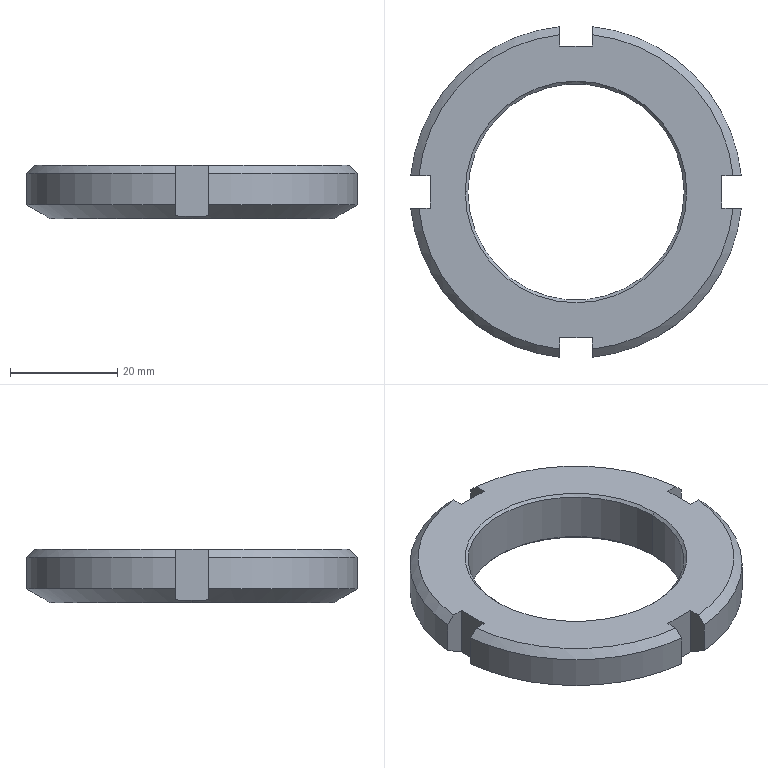Part | SolidWorks | features Chamfer 3, CirPattern 1, Cut 1, Extrusion 1 | 1 solid | 30 faces | box 61.709 x 61.709 x 10 mm | volume 15331 mm3 | plane 14 | cone 10 | cylinder 6 | commonest cylinder face diameters 62 x4 40.376 x2
STEP:
#1=CARTESIAN_POINT('',(-20.188,0.,9.5));
#2=VERTEX_POINT('',#1);
#3=CARTESIAN_POINT('',(20.188,0.,9.5));
#4=VERTEX_POINT('',#3);
#5=CARTESIAN_POINT('',(0.,0.,9.5));
#6=DIRECTION('',(0.,0.,1.));
#7=DIRECTION('',(1.,0.,0.));
#8=AXIS2_PLACEMENT_3D('',#5,#6,#7);
#9=CIRCLE('',#8,20.188);
#10=EDGE_CURVE('',#2,#4,#9,.T.);
#11=ORIENTED_EDGE('',*,*,#10,.F.);
#12=CARTESIAN_POINT('',(-20.688,0.,10.));
#13=VERTEX_POINT('',#12);
#14=CARTESIAN_POINT('',(-20.188,0.,9.5));
#15=DIRECTION('',(-0.7071,0.,0.7071));
#16=VECTOR('',#15,1000.);
#17=LINE('',#14,#16);
#18=EDGE_CURVE('',#2,#13,#17,.T.);
#19=ORIENTED_EDGE('',*,*,#18,.T.);
#20=CARTESIAN_POINT('',(20.688,0.,10.));
#21=VERTEX_POINT('',#20);
#22=CARTESIAN_POINT('',(0.,0.,10.));
#23=DIRECTION('',(0.,0.,-1.));
#24=DIRECTION('',(1.,0.,0.));
#25=AXIS2_PLACEMENT_3D('',#22,#23,#24);
#26=CIRCLE('',#25,20.688);
#27=EDGE_CURVE('',#21,#13,#26,.T.);
#28=ORIENTED_EDGE('',*,*,#27,.F.);
#29=CARTESIAN_POINT('',(20.188,0.,9.5));
#30=DIRECTION('',(0.7071,0.,0.7071));
#31=VECTOR('',#30,1000.);
#32=LINE('',#29,#31);
#33=EDGE_CURVE('',#4,#21,#32,.T.);
#34=ORIENTED_EDGE('',*,*,#33,.F.);
#35=EDGE_LOOP('',(#11,#19,#28,#34));
#36=FACE_OUTER_BOUND('',#35,.T.);
#37=CARTESIAN_POINT('',(0.,0.,9.5));
#38=DIRECTION('',(0.,0.,1.));
#39=DIRECTION('',(1.,0.,0.));
#40=AXIS2_PLACEMENT_3D('',#37,#38,#39);
#41=CONICAL_SURFACE('',#40,20.188,0.7854);
#42=ADVANCED_FACE('',(#36),#41,.F.);
#43=CARTESIAN_POINT('',(20.188,0.,0.5));
#44=VERTEX_POINT('',#43);
#45=CARTESIAN_POINT('',(-20.188,0.,0.5));
#46=VERTEX_POINT('',#45);
#47=CARTESIAN_POINT('',(0.,0.,0.5));
#48=DIRECTION('',(0.,0.,-1.));
#49=DIRECTION('',(1.,0.,0.));
#50=AXIS2_PLACEMENT_3D('',#47,#48,#49);
#51=CIRCLE('',#50,20.188);
#52=EDGE_CURVE('',#44,#46,#51,.T.);
#53=ORIENTED_EDGE('',*,*,#52,.F.);
#54=CARTESIAN_POINT('',(20.688,0.,0.));
#55=VERTEX_POINT('',#54);
#56=CARTESIAN_POINT('',(20.688,0.,0.));
#57=DIRECTION('',(0.7071,0.,-0.7071));
#58=VECTOR('',#57,1000.);
#59=LINE('',#56,#58);
#60=EDGE_CURVE('',#44,#55,#59,.T.);
#61=ORIENTED_EDGE('',*,*,#60,.T.);
#62=CARTESIAN_POINT('',(-20.688,0.,0.));
#63=VERTEX_POINT('',#62);
#64=CARTESIAN_POINT('',(0.,0.,0.));
#65=DIRECTION('',(0.,0.,1.));
#66=DIRECTION('',(1.,0.,0.));
#67=AXIS2_PLACEMENT_3D('',#64,#65,#66);
#68=CIRCLE('',#67,20.688);
#69=EDGE_CURVE('',#63,#55,#68,.T.);
#70=ORIENTED_EDGE('',*,*,#69,.F.);
#71=CARTESIAN_POINT('',(-20.688,0.,0.));
#72=DIRECTION('',(-0.7071,0.,-0.7071));
#73=VECTOR('',#72,1000.);
#74=LINE('',#71,#73);
#75=EDGE_CURVE('',#46,#63,#74,.T.);
#76=ORIENTED_EDGE('',*,*,#75,.F.);
#77=EDGE_LOOP('',(#53,#61,#70,#76));
#78=FACE_OUTER_BOUND('',#77,.T.);
#79=CARTESIAN_POINT('',(0.,0.,0.));
#80=DIRECTION('',(0.,0.,-1.));
#81=DIRECTION('',(-1.,0.,0.));
#82=AXIS2_PLACEMENT_3D('',#79,#80,#81);
#83=CONICAL_SURFACE('',#82,20.688,0.7854);
#84=ADVANCED_FACE('',(#78),#83,.F.);
#85=CARTESIAN_POINT('',(-26.5,0.,0.));
#86=VERTEX_POINT('',#85);
#87=CARTESIAN_POINT('',(26.5,0.,0.));
#88=VERTEX_POINT('',#87);
#89=CARTESIAN_POINT('',(0.,0.,0.));
#90=DIRECTION('',(0.,0.,-1.));
#91=DIRECTION('',(1.,0.,0.));
#92=AXIS2_PLACEMENT_3D('',#89,#90,#91);
#93=CIRCLE('',#92,26.5);
#94=EDGE_CURVE('',#86,#88,#93,.T.);
#95=ORIENTED_EDGE('',*,*,#94,.F.);
#96=CARTESIAN_POINT('',(-27.254,0.,0.4356));
#97=VERTEX_POINT('',#96);
#98=CARTESIAN_POINT('',(-31.,0.,2.598));
#99=DIRECTION('',(-0.866,0.,0.5));
#100=VECTOR('',#99,1000.);
#101=LINE('',#98,#100);
#102=EDGE_CURVE('',#86,#97,#101,.T.);
#103=ORIENTED_EDGE('',*,*,#102,.T.);
#104=CARTESIAN_POINT('',(-27.254,3.,0.5306));
#105=VERTEX_POINT('',#104);
#106=CARTESIAN_POINT('',(-27.254,3.,0.5306));
#107=CARTESIAN_POINT('',(-27.254,2.003,0.4677));
#108=CARTESIAN_POINT('',(-27.254,1.003,0.4356));
#109=CARTESIAN_POINT('',(-27.254,0.,0.4356));
#110=B_SPLINE_CURVE_WITH_KNOTS('',3,(#106,#107,#108,#109),.UNSPECIFIED.,.F.,.F.,(4,4),(0.007971,0.01097),.UNSPECIFIED.);
#111=EDGE_CURVE('',#105,#97,#110,.T.);
#112=ORIENTED_EDGE('',*,*,#111,.F.);
#113=CARTESIAN_POINT('',(-30.854,3.,2.598));
#114=VERTEX_POINT('',#113);
#115=CARTESIAN_POINT('',(-30.854,3.,2.598));
#116=CARTESIAN_POINT('',(-30.648,3.,2.48));
#117=CARTESIAN_POINT('',(-30.442,3.,2.361));
#118=CARTESIAN_POINT('',(-30.236,3.,2.242));
#119=CARTESIAN_POINT('',(-29.242,3.,1.672));
#120=CARTESIAN_POINT('',(-28.248,3.,1.101));
#121=CARTESIAN_POINT('',(-27.254,3.,0.5306));
#122=B_SPLINE_CURVE_WITH_KNOTS('',3,(#115,#116,#117,#118,#119,#120,#121),.UNSPECIFIED.,.F.,.F.,(4,3,4),(0.007772,0.008485,0.01192),.UNSPECIFIED.);
#123=EDGE_CURVE('',#114,#105,#122,.T.);
#124=ORIENTED_EDGE('',*,*,#123,.F.);
#125=CARTESIAN_POINT('',(-3.,30.854,2.598));
#126=VERTEX_POINT('',#125);
#127=CARTESIAN_POINT('',(0.,0.,2.598));
#128=DIRECTION('',(0.,0.,1.));
#129=DIRECTION('',(1.,0.,0.));
#130=AXIS2_PLACEMENT_3D('',#127,#128,#129);
#131=CIRCLE('',#130,31.);
#132=EDGE_CURVE('',#126,#114,#131,.T.);
#133=ORIENTED_EDGE('',*,*,#132,.F.);
#134=CARTESIAN_POINT('',(-3.,27.254,0.5306));
#135=VERTEX_POINT('',#134);
#136=CARTESIAN_POINT('',(-3.,27.254,0.5306));
#137=CARTESIAN_POINT('',(-3.,28.455,1.219));
#138=CARTESIAN_POINT('',(-3.,29.655,1.909));
#139=CARTESIAN_POINT('',(-3.,30.854,2.598));
#140=B_SPLINE_CURVE_WITH_KNOTS('',3,(#136,#137,#138,#139),.UNSPECIFIED.,.F.,.F.,(4,4),(0.008036,0.01219),.UNSPECIFIED.);
#141=EDGE_CURVE('',#135,#126,#140,.T.);
#142=ORIENTED_EDGE('',*,*,#141,.F.);
#143=CARTESIAN_POINT('',(3.,27.254,0.5306));
#144=VERTEX_POINT('',#143);
#145=CARTESIAN_POINT('',(3.,27.254,0.5306));
#146=CARTESIAN_POINT('',(2.005,27.254,0.4678));
#147=CARTESIAN_POINT('',(1.008,27.254,0.4358));
#148=CARTESIAN_POINT('',(-0.9926,27.254,0.4354));
#149=CARTESIAN_POINT('',(-1.998,27.254,0.4674));
#150=CARTESIAN_POINT('',(-3.,27.254,0.5306));
#151=B_SPLINE_CURVE_WITH_KNOTS('',3,(#145,#146,#147,#148,#149,#150),.UNSPECIFIED.,.F.,.F.,(4,2,4),(0.007971,0.01096,0.01395),.UNSPECIFIED.);
#152=EDGE_CURVE('',#144,#135,#151,.T.);
#153=ORIENTED_EDGE('',*,*,#152,.F.);
#154=CARTESIAN_POINT('',(3.,30.854,2.598));
#155=VERTEX_POINT('',#154);
#156=CARTESIAN_POINT('',(3.,30.854,2.598));
#157=CARTESIAN_POINT('',(3.,29.655,1.909));
#158=CARTESIAN_POINT('',(3.,28.455,1.219));
#159=CARTESIAN_POINT('',(3.,27.254,0.5306));
#160=B_SPLINE_CURVE_WITH_KNOTS('',3,(#156,#157,#158,#159),.UNSPECIFIED.,.F.,.F.,(4,4),(0.004783,0.008935),.UNSPECIFIED.);
#161=EDGE_CURVE('',#155,#144,#160,.T.);
#162=ORIENTED_EDGE('',*,*,#161,.F.);
#163=CARTESIAN_POINT('',(30.854,3.,2.598));
#164=VERTEX_POINT('',#163);
#165=CARTESIAN_POINT('',(0.,0.,2.598));
#166=DIRECTION('',(0.,0.,1.));
#167=DIRECTION('',(1.,0.,0.));
#168=AXIS2_PLACEMENT_3D('',#165,#166,#167);
#169=CIRCLE('',#168,31.);
#170=EDGE_CURVE('',#164,#155,#169,.T.);
#171=ORIENTED_EDGE('',*,*,#170,.F.);
#172=CARTESIAN_POINT('',(27.254,3.,0.5306));
#173=VERTEX_POINT('',#172);
#174=CARTESIAN_POINT('',(27.254,3.,0.5306));
#175=CARTESIAN_POINT('',(28.455,3.,1.219));
#176=CARTESIAN_POINT('',(29.655,3.,1.909));
#177=CARTESIAN_POINT('',(30.854,3.,2.598));
#178=B_SPLINE_CURVE_WITH_KNOTS('',3,(#174,#175,#176,#177),.UNSPECIFIED.,.F.,.F.,(4,4),(0.008036,0.01219),.UNSPECIFIED.);
#179=EDGE_CURVE('',#173,#164,#178,.T.);
#180=ORIENTED_EDGE('',*,*,#179,.F.);
#181=CARTESIAN_POINT('',(27.254,0.,0.4356));
#182=VERTEX_POINT('',#181);
#183=CARTESIAN_POINT('',(27.254,0.,0.4356));
#184=CARTESIAN_POINT('',(27.254,1.003,0.4356));
#185=CARTESIAN_POINT('',(27.254,2.003,0.4677));
#186=CARTESIAN_POINT('',(27.254,3.,0.5306));
#187=B_SPLINE_CURVE_WITH_KNOTS('',3,(#183,#184,#185,#186),.UNSPECIFIED.,.F.,.F.,(4,4),(0.01544,0.01844),.UNSPECIFIED.);
#188=EDGE_CURVE('',#182,#173,#187,.T.);
#189=ORIENTED_EDGE('',*,*,#188,.F.);
#190=CARTESIAN_POINT('',(31.,0.,2.598));
#191=DIRECTION('',(0.866,0.,0.5));
#192=VECTOR('',#191,1000.);
#193=LINE('',#190,#192);
#194=EDGE_CURVE('',#88,#182,#193,.T.);
#195=ORIENTED_EDGE('',*,*,#194,.F.);
#196=EDGE_LOOP('',(#95,#103,#112,#124,#133,#142,#153,#162,#171,#180,#189,#195));
#197=FACE_OUTER_BOUND('',#196,.T.);
#198=CARTESIAN_POINT('',(0.,0.,2.598));
#199=DIRECTION('',(0.,0.,1.));
#200=DIRECTION('',(1.,0.,0.));
#201=AXIS2_PLACEMENT_3D('',#198,#199,#200);
#202=CONICAL_SURFACE('',#201,31.,1.047);
#203=ADVANCED_FACE('',(#197),#202,.T.);
#204=ORIENTED_EDGE('',*,*,#10,.T.);
#205=CARTESIAN_POINT('',(20.188,0.,10.));
#206=DIRECTION('',(0.,0.,-1.));
#207=VECTOR('',#206,1000.);
#208=LINE('',#205,#207);
#209=EDGE_CURVE('',#4,#44,#208,.T.);
#210=ORIENTED_EDGE('',*,*,#209,.T.);
#211=ORIENTED_EDGE('',*,*,#52,.T.);
#212=CARTESIAN_POINT('',(-20.188,0.,10.));
#213=DIRECTION('',(0.,0.,-1.));
#214=VECTOR('',#213,1000.);
#215=LINE('',#212,#214);
#216=EDGE_CURVE('',#2,#46,#215,.T.);
#217=ORIENTED_EDGE('',*,*,#216,.F.);
#218=EDGE_LOOP('',(#204,#210,#211,#217));
#219=FACE_OUTER_BOUND('',#218,.T.);
#220=CARTESIAN_POINT('',(0.,0.,10.));
#221=DIRECTION('',(0.,0.,-1.));
#222=DIRECTION('',(-1.,0.,0.));
#223=AXIS2_PLACEMENT_3D('',#220,#221,#222);
#224=CYLINDRICAL_SURFACE('',#223,20.188);
#225=ADVANCED_FACE('',(#219),#224,.F.);
#226=CARTESIAN_POINT('',(3.,30.854,8.5));
#227=VERTEX_POINT('',#226);
#228=CARTESIAN_POINT('',(30.854,3.,8.5));
#229=VERTEX_POINT('',#228);
#230=CARTESIAN_POINT('',(0.,0.,8.5));
#231=DIRECTION('',(0.,0.,-1.));
#232=DIRECTION('',(1.,0.,0.));
#233=AXIS2_PLACEMENT_3D('',#230,#231,#232);
#234=CIRCLE('',#233,31.);
#235=EDGE_CURVE('',#227,#229,#234,.T.);
#236=ORIENTED_EDGE('',*,*,#235,.T.);
#237=CARTESIAN_POINT('',(30.854,3.,0.));
#238=DIRECTION('',(0.,0.,1.));
#239=VECTOR('',#238,1000.);
#240=LINE('',#237,#239);
#241=EDGE_CURVE('',#164,#229,#240,.T.);
#242=ORIENTED_EDGE('',*,*,#241,.F.);
#243=ORIENTED_EDGE('',*,*,#170,.T.);
#244=CARTESIAN_POINT('',(3.,30.854,0.));
#245=DIRECTION('',(0.,0.,1.));
#246=VECTOR('',#245,1000.);
#247=LINE('',#244,#246);
#248=EDGE_CURVE('',#155,#227,#247,.T.);
#249=ORIENTED_EDGE('',*,*,#248,.T.);
#250=EDGE_LOOP('',(#236,#242,#243,#249));
#251=FACE_OUTER_BOUND('',#250,.T.);
#252=CARTESIAN_POINT('',(0.,0.,10.));
#253=DIRECTION('',(0.,0.,-1.));
#254=DIRECTION('',(-1.,0.,0.));
#255=AXIS2_PLACEMENT_3D('',#252,#253,#254);
#256=CYLINDRICAL_SURFACE('',#255,31.);
#257=ADVANCED_FACE('',(#251),#256,.T.);
#258=CARTESIAN_POINT('',(29.347,3.,10.));
#259=VERTEX_POINT('',#258);
#260=CARTESIAN_POINT('',(30.854,3.,8.5));
#261=CARTESIAN_POINT('',(30.441,3.,8.912));
#262=CARTESIAN_POINT('',(30.027,3.,9.323));
#263=CARTESIAN_POINT('',(29.614,3.,9.735));
#264=CARTESIAN_POINT('',(29.525,3.,9.823));
#265=CARTESIAN_POINT('',(29.436,3.,9.912));
#266=CARTESIAN_POINT('',(29.347,3.,10.));
#267=B_SPLINE_CURVE_WITH_KNOTS('',3,(#260,#261,#262,#263,#264,#265,#266),.UNSPECIFIED.,.F.,.F.,(4,3,4),(0.006071,0.007821,0.008198),.UNSPECIFIED.);
#268=EDGE_CURVE('',#229,#259,#267,.T.);
#269=ORIENTED_EDGE('',*,*,#268,.F.);
#270=ORIENTED_EDGE('',*,*,#235,.F.);
#271=CARTESIAN_POINT('',(3.,29.347,10.));
#272=VERTEX_POINT('',#271);
#273=CARTESIAN_POINT('',(3.,29.347,10.));
#274=CARTESIAN_POINT('',(3.,29.436,9.912));
#275=CARTESIAN_POINT('',(3.,29.525,9.823));
#276=CARTESIAN_POINT('',(3.,29.614,9.735));
#277=CARTESIAN_POINT('',(3.,30.027,9.323));
#278=CARTESIAN_POINT('',(3.,30.441,8.912));
#279=CARTESIAN_POINT('',(3.,30.854,8.5));
#280=B_SPLINE_CURVE_WITH_KNOTS('',3,(#273,#274,#275,#276,#277,#278,#279),.UNSPECIFIED.,.F.,.F.,(4,3,4),(0.007445,0.007821,0.009572),.UNSPECIFIED.);
#281=EDGE_CURVE('',#272,#227,#280,.T.);
#282=ORIENTED_EDGE('',*,*,#281,.F.);
#283=CARTESIAN_POINT('',(0.,0.,10.));
#284=DIRECTION('',(0.,0.,1.));
#285=DIRECTION('',(1.,0.,0.));
#286=AXIS2_PLACEMENT_3D('',#283,#284,#285);
#287=CIRCLE('',#286,29.5);
#288=EDGE_CURVE('',#259,#272,#287,.T.);
#289=ORIENTED_EDGE('',*,*,#288,.F.);
#290=EDGE_LOOP('',(#269,#270,#282,#289));
#291=FACE_OUTER_BOUND('',#290,.T.);
#292=CARTESIAN_POINT('',(0.,0.,10.));
#293=DIRECTION('',(0.,0.,-1.));
#294=DIRECTION('',(-1.,0.,0.));
#295=AXIS2_PLACEMENT_3D('',#292,#293,#294);
#296=CONICAL_SURFACE('',#295,29.5,0.7854);
#297=ADVANCED_FACE('',(#291),#296,.T.);
#298=CARTESIAN_POINT('',(-30.854,3.,8.5));
#299=VERTEX_POINT('',#298);
#300=CARTESIAN_POINT('',(-3.,30.854,8.5));
#301=VERTEX_POINT('',#300);
#302=CARTESIAN_POINT('',(0.,0.,8.5));
#303=DIRECTION('',(0.,0.,-1.));
#304=DIRECTION('',(1.,0.,0.));
#305=AXIS2_PLACEMENT_3D('',#302,#303,#304);
#306=CIRCLE('',#305,31.);
#307=EDGE_CURVE('',#299,#301,#306,.T.);
#308=ORIENTED_EDGE('',*,*,#307,.T.);
#309=CARTESIAN_POINT('',(-3.,30.854,0.));
#310=DIRECTION('',(0.,0.,1.));
#311=VECTOR('',#310,1000.);
#312=LINE('',#309,#311);
#313=EDGE_CURVE('',#126,#301,#312,.T.);
#314=ORIENTED_EDGE('',*,*,#313,.F.);
#315=ORIENTED_EDGE('',*,*,#132,.T.);
#316=CARTESIAN_POINT('',(-30.854,3.,0.));
#317=DIRECTION('',(0.,0.,1.));
#318=VECTOR('',#317,1000.);
#319=LINE('',#316,#318);
#320=EDGE_CURVE('',#114,#299,#319,.T.);
#321=ORIENTED_EDGE('',*,*,#320,.T.);
#322=EDGE_LOOP('',(#308,#314,#315,#321));
#323=FACE_OUTER_BOUND('',#322,.T.);
#324=CARTESIAN_POINT('',(0.,0.,10.));
#325=DIRECTION('',(0.,0.,-1.));
#326=DIRECTION('',(-1.,0.,0.));
#327=AXIS2_PLACEMENT_3D('',#324,#325,#326);
#328=CYLINDRICAL_SURFACE('',#327,31.);
#329=ADVANCED_FACE('',(#323),#328,.T.);
#330=CARTESIAN_POINT('',(-3.,29.347,10.));
#331=VERTEX_POINT('',#330);
#332=CARTESIAN_POINT('',(-3.,30.854,8.5));
#333=CARTESIAN_POINT('',(-3.,30.441,8.912));
#334=CARTESIAN_POINT('',(-3.,30.027,9.323));
#335=CARTESIAN_POINT('',(-3.,29.614,9.735));
#336=CARTESIAN_POINT('',(-3.,29.525,9.823));
#337=CARTESIAN_POINT('',(-3.,29.436,9.912));
#338=CARTESIAN_POINT('',(-3.,29.347,10.));
#339=B_SPLINE_CURVE_WITH_KNOTS('',3,(#332,#333,#334,#335,#336,#337,#338),.UNSPECIFIED.,.F.,.F.,(4,3,4),(0.006071,0.007821,0.008198),.UNSPECIFIED.);
#340=EDGE_CURVE('',#301,#331,#339,.T.);
#341=ORIENTED_EDGE('',*,*,#340,.F.);
#342=ORIENTED_EDGE('',*,*,#307,.F.);
#343=CARTESIAN_POINT('',(-29.347,3.,10.));
#344=VERTEX_POINT('',#343);
#345=CARTESIAN_POINT('',(-29.347,3.,10.));
#346=CARTESIAN_POINT('',(-29.712,3.,9.637));
#347=CARTESIAN_POINT('',(-30.076,3.,9.274));
#348=CARTESIAN_POINT('',(-30.441,3.,8.912));
#349=CARTESIAN_POINT('',(-30.579,3.,8.774));
#350=CARTESIAN_POINT('',(-30.717,3.,8.637));
#351=CARTESIAN_POINT('',(-30.854,3.,8.5));
#352=B_SPLINE_CURVE_WITH_KNOTS('',3,(#345,#346,#347,#348,#349,#350,#351),.UNSPECIFIED.,.F.,.F.,(4,3,4),(0.006278,0.007821,0.008405),.UNSPECIFIED.);
#353=EDGE_CURVE('',#344,#299,#352,.T.);
#354=ORIENTED_EDGE('',*,*,#353,.F.);
#355=CARTESIAN_POINT('',(0.,0.,10.));
#356=DIRECTION('',(0.,0.,1.));
#357=DIRECTION('',(1.,0.,0.));
#358=AXIS2_PLACEMENT_3D('',#355,#356,#357);
#359=CIRCLE('',#358,29.5);
#360=EDGE_CURVE('',#331,#344,#359,.T.);
#361=ORIENTED_EDGE('',*,*,#360,.F.);
#362=EDGE_LOOP('',(#341,#342,#354,#361));
#363=FACE_OUTER_BOUND('',#362,.T.);
#364=CARTESIAN_POINT('',(0.,0.,10.));
#365=DIRECTION('',(0.,0.,-1.));
#366=DIRECTION('',(-1.,0.,0.));
#367=AXIS2_PLACEMENT_3D('',#364,#365,#366);
#368=CONICAL_SURFACE('',#367,29.5,0.7854);
#369=ADVANCED_FACE('',(#363),#368,.T.);
#370=CARTESIAN_POINT('',(-3.,-30.854,8.5));
#371=VERTEX_POINT('',#370);
#372=CARTESIAN_POINT('',(-30.854,-3.,8.5));
#373=VERTEX_POINT('',#372);
#374=CARTESIAN_POINT('',(0.,0.,8.5));
#375=DIRECTION('',(0.,0.,-1.));
#376=DIRECTION('',(1.,0.,0.));
#377=AXIS2_PLACEMENT_3D('',#374,#375,#376);
#378=CIRCLE('',#377,31.);
#379=EDGE_CURVE('',#371,#373,#378,.T.);
#380=ORIENTED_EDGE('',*,*,#379,.T.);
#381=CARTESIAN_POINT('',(-30.854,-3.,2.598));
#382=VERTEX_POINT('',#381);
#383=CARTESIAN_POINT('',(-30.854,-3.,0.));
#384=DIRECTION('',(0.,0.,1.));
#385=VECTOR('',#384,1000.);
#386=LINE('',#383,#385);
#387=EDGE_CURVE('',#382,#373,#386,.T.);
#388=ORIENTED_EDGE('',*,*,#387,.F.);
#389=CARTESIAN_POINT('',(-3.,-30.854,2.598));
#390=VERTEX_POINT('',#389);
#391=CARTESIAN_POINT('',(0.,0.,2.598));
#392=DIRECTION('',(0.,0.,1.));
#393=DIRECTION('',(1.,0.,0.));
#394=AXIS2_PLACEMENT_3D('',#391,#392,#393);
#395=CIRCLE('',#394,31.);
#396=EDGE_CURVE('',#382,#390,#395,.T.);
#397=ORIENTED_EDGE('',*,*,#396,.T.);
#398=CARTESIAN_POINT('',(-3.,-30.854,0.));
#399=DIRECTION('',(0.,0.,1.));
#400=VECTOR('',#399,1000.);
#401=LINE('',#398,#400);
#402=EDGE_CURVE('',#390,#371,#401,.T.);
#403=ORIENTED_EDGE('',*,*,#402,.T.);
#404=EDGE_LOOP('',(#380,#388,#397,#403));
#405=FACE_OUTER_BOUND('',#404,.T.);
#406=CARTESIAN_POINT('',(0.,0.,10.));
#407=DIRECTION('',(0.,0.,-1.));
#408=DIRECTION('',(-1.,0.,0.));
#409=AXIS2_PLACEMENT_3D('',#406,#407,#408);
#410=CYLINDRICAL_SURFACE('',#409,31.);
#411=ADVANCED_FACE('',(#405),#410,.T.);
#412=CARTESIAN_POINT('',(-29.347,-3.,10.));
#413=VERTEX_POINT('',#412);
#414=CARTESIAN_POINT('',(-30.854,-3.,8.5));
#415=CARTESIAN_POINT('',(-30.717,-3.,8.637));
#416=CARTESIAN_POINT('',(-30.579,-3.,8.774));
#417=CARTESIAN_POINT('',(-30.441,-3.,8.912));
#418=CARTESIAN_POINT('',(-30.076,-3.,9.274));
#419=CARTESIAN_POINT('',(-29.712,-3.,9.637));
#420=CARTESIAN_POINT('',(-29.347,-3.,10.));
#421=B_SPLINE_CURVE_WITH_KNOTS('',3,(#414,#415,#416,#417,#418,#419,#420),.UNSPECIFIED.,.F.,.F.,(4,3,4),(0.007238,0.007821,0.009365),.UNSPECIFIED.);
#422=EDGE_CURVE('',#373,#413,#421,.T.);
#423=ORIENTED_EDGE('',*,*,#422,.F.);
#424=ORIENTED_EDGE('',*,*,#379,.F.);
#425=CARTESIAN_POINT('',(-3.,-29.347,10.));
#426=VERTEX_POINT('',#425);
#427=CARTESIAN_POINT('',(-3.,-29.347,10.));
#428=CARTESIAN_POINT('',(-3.,-29.712,9.637));
#429=CARTESIAN_POINT('',(-3.,-30.076,9.274));
#430=CARTESIAN_POINT('',(-3.,-30.441,8.912));
#431=CARTESIAN_POINT('',(-3.,-30.579,8.774));
#432=CARTESIAN_POINT('',(-3.,-30.717,8.637));
#433=CARTESIAN_POINT('',(-3.,-30.854,8.5));
#434=B_SPLINE_CURVE_WITH_KNOTS('',3,(#427,#428,#429,#430,#431,#432,#433),.UNSPECIFIED.,.F.,.F.,(4,3,4),(0.006278,0.007821,0.008405),.UNSPECIFIED.);
#435=EDGE_CURVE('',#426,#371,#434,.T.);
#436=ORIENTED_EDGE('',*,*,#435,.F.);
#437=CARTESIAN_POINT('',(0.,0.,10.));
#438=DIRECTION('',(0.,0.,1.));
#439=DIRECTION('',(1.,0.,0.));
#440=AXIS2_PLACEMENT_3D('',#437,#438,#439);
#441=CIRCLE('',#440,29.5);
#442=EDGE_CURVE('',#413,#426,#441,.T.);
#443=ORIENTED_EDGE('',*,*,#442,.F.);
#444=EDGE_LOOP('',(#423,#424,#436,#443));
#445=FACE_OUTER_BOUND('',#444,.T.);
#446=CARTESIAN_POINT('',(0.,0.,10.));
#447=DIRECTION('',(0.,0.,-1.));
#448=DIRECTION('',(-1.,0.,0.));
#449=AXIS2_PLACEMENT_3D('',#446,#447,#448);
#450=CONICAL_SURFACE('',#449,29.5,0.7854);
#451=ADVANCED_FACE('',(#445),#450,.T.);
#452=ORIENTED_EDGE('',*,*,#27,.T.);
#453=CARTESIAN_POINT('',(0.,0.,10.));
#454=DIRECTION('',(0.,0.,-1.));
#455=DIRECTION('',(1.,0.,0.));
#456=AXIS2_PLACEMENT_3D('',#453,#454,#455);
#457=CIRCLE('',#456,20.688);
#458=EDGE_CURVE('',#13,#21,#457,.T.);
#459=ORIENTED_EDGE('',*,*,#458,.T.);
#460=EDGE_LOOP('',(#452,#459));
#461=FACE_BOUND('',#460,.T.);
#462=CARTESIAN_POINT('',(27.254,3.,10.));
#463=VERTEX_POINT('',#462);
#464=CARTESIAN_POINT('',(27.254,3.,10.));
#465=DIRECTION('',(-1.,0.,0.));
#466=VECTOR('',#465,1000.);
#467=LINE('',#464,#466);
#468=EDGE_CURVE('',#259,#463,#467,.T.);
#469=ORIENTED_EDGE('',*,*,#468,.F.);
#470=ORIENTED_EDGE('',*,*,#288,.T.);
#471=CARTESIAN_POINT('',(3.,27.254,10.));
#472=VERTEX_POINT('',#471);
#473=CARTESIAN_POINT('',(3.,27.254,10.));
#474=DIRECTION('',(0.,1.,0.));
#475=VECTOR('',#474,1000.);
#476=LINE('',#473,#475);
#477=EDGE_CURVE('',#472,#272,#476,.T.);
#478=ORIENTED_EDGE('',*,*,#477,.F.);
#479=CARTESIAN_POINT('',(-3.,27.254,10.));
#480=VERTEX_POINT('',#479);
#481=CARTESIAN_POINT('',(3.,27.254,10.));
#482=DIRECTION('',(1.,0.,0.));
#483=VECTOR('',#482,1000.);
#484=LINE('',#481,#483);
#485=EDGE_CURVE('',#480,#472,#484,.T.);
#486=ORIENTED_EDGE('',*,*,#485,.F.);
#487=CARTESIAN_POINT('',(-3.,27.254,10.));
#488=DIRECTION('',(0.,-1.,0.));
#489=VECTOR('',#488,1000.);
#490=LINE('',#487,#489);
#491=EDGE_CURVE('',#331,#480,#490,.T.);
#492=ORIENTED_EDGE('',*,*,#491,.F.);
#493=ORIENTED_EDGE('',*,*,#360,.T.);
#494=CARTESIAN_POINT('',(-27.254,3.,10.));
#495=VERTEX_POINT('',#494);
#496=CARTESIAN_POINT('',(-27.254,3.,10.));
#497=DIRECTION('',(-1.,0.,0.));
#498=VECTOR('',#497,1000.);
#499=LINE('',#496,#498);
#500=EDGE_CURVE('',#495,#344,#499,.T.);
#501=ORIENTED_EDGE('',*,*,#500,.F.);
#502=CARTESIAN_POINT('',(-27.254,-3.,10.));
#503=VERTEX_POINT('',#502);
#504=CARTESIAN_POINT('',(-27.254,3.,10.));
#505=DIRECTION('',(0.,1.,0.));
#506=VECTOR('',#505,1000.);
#507=LINE('',#504,#506);
#508=EDGE_CURVE('',#503,#495,#507,.T.);
#509=ORIENTED_EDGE('',*,*,#508,.F.);
#510=CARTESIAN_POINT('',(-27.254,-3.,10.));
#511=DIRECTION('',(1.,0.,0.));
#512=VECTOR('',#511,1000.);
#513=LINE('',#510,#512);
#514=EDGE_CURVE('',#413,#503,#513,.T.);
#515=ORIENTED_EDGE('',*,*,#514,.F.);
#516=ORIENTED_EDGE('',*,*,#442,.T.);
#517=CARTESIAN_POINT('',(-3.,-27.254,10.));
#518=VERTEX_POINT('',#517);
#519=CARTESIAN_POINT('',(-3.,-27.254,10.));
#520=DIRECTION('',(0.,-1.,0.));
#521=VECTOR('',#520,1000.);
#522=LINE('',#519,#521);
#523=EDGE_CURVE('',#518,#426,#522,.T.);
#524=ORIENTED_EDGE('',*,*,#523,.F.);
#525=CARTESIAN_POINT('',(3.,-27.254,10.));
#526=VERTEX_POINT('',#525);
#527=CARTESIAN_POINT('',(-3.,-27.254,10.));
#528=DIRECTION('',(-1.,0.,0.));
#529=VECTOR('',#528,1000.);
#530=LINE('',#527,#529);
#531=EDGE_CURVE('',#526,#518,#530,.T.);
#532=ORIENTED_EDGE('',*,*,#531,.F.);
#533=CARTESIAN_POINT('',(3.,-29.347,10.));
#534=VERTEX_POINT('',#533);
#535=CARTESIAN_POINT('',(3.,-27.254,10.));
#536=DIRECTION('',(0.,1.,0.));
#537=VECTOR('',#536,1000.);
#538=LINE('',#535,#537);
#539=EDGE_CURVE('',#534,#526,#538,.T.);
#540=ORIENTED_EDGE('',*,*,#539,.F.);
#541=CARTESIAN_POINT('',(29.347,-3.,10.));
#542=VERTEX_POINT('',#541);
#543=CARTESIAN_POINT('',(0.,0.,10.));
#544=DIRECTION('',(0.,0.,1.));
#545=DIRECTION('',(1.,0.,0.));
#546=AXIS2_PLACEMENT_3D('',#543,#544,#545);
#547=CIRCLE('',#546,29.5);
#548=EDGE_CURVE('',#534,#542,#547,.T.);
#549=ORIENTED_EDGE('',*,*,#548,.T.);
#550=CARTESIAN_POINT('',(27.254,-3.,10.));
#551=VERTEX_POINT('',#550);
#552=CARTESIAN_POINT('',(27.254,-3.,10.));
#553=DIRECTION('',(1.,0.,0.));
#554=VECTOR('',#553,1000.);
#555=LINE('',#552,#554);
#556=EDGE_CURVE('',#551,#542,#555,.T.);
#557=ORIENTED_EDGE('',*,*,#556,.F.);
#558=CARTESIAN_POINT('',(27.254,-3.,10.));
#559=DIRECTION('',(0.,-1.,0.));
#560=VECTOR('',#559,1000.);
#561=LINE('',#558,#560);
#562=EDGE_CURVE('',#463,#551,#561,.T.);
#563=ORIENTED_EDGE('',*,*,#562,.F.);
#564=EDGE_LOOP('',(#469,#470,#478,#486,#492,#493,#501,#509,#515,#516,#524,#532,#540,#549,#557,#563));
#565=FACE_OUTER_BOUND('',#564,.T.);
#566=CARTESIAN_POINT('',(0.,0.,10.));
#567=DIRECTION('',(0.,0.,1.));
#568=DIRECTION('',(1.,0.,0.));
#569=AXIS2_PLACEMENT_3D('',#566,#567,#568);
#570=PLANE('',#569);
#571=ADVANCED_FACE('',(#461,#565),#570,.T.);
#572=ORIENTED_EDGE('',*,*,#69,.T.);
#573=CARTESIAN_POINT('',(0.,0.,0.));
#574=DIRECTION('',(0.,0.,1.));
#575=DIRECTION('',(1.,0.,0.));
#576=AXIS2_PLACEMENT_3D('',#573,#574,#575);
#577=CIRCLE('',#576,20.688);
#578=EDGE_CURVE('',#55,#63,#577,.T.);
#579=ORIENTED_EDGE('',*,*,#578,.T.);
#580=EDGE_LOOP('',(#572,#579));
#581=FACE_BOUND('',#580,.T.);
#582=CARTESIAN_POINT('',(0.,0.,0.));
#583=DIRECTION('',(0.,0.,-1.));
#584=DIRECTION('',(1.,0.,0.));
#585=AXIS2_PLACEMENT_3D('',#582,#583,#584);
#586=CIRCLE('',#585,26.5);
#587=EDGE_CURVE('',#88,#86,#586,.T.);
#588=ORIENTED_EDGE('',*,*,#587,.T.);
#589=ORIENTED_EDGE('',*,*,#94,.T.);
#590=EDGE_LOOP('',(#588,#589));
#591=FACE_OUTER_BOUND('',#590,.T.);
#592=CARTESIAN_POINT('',(0.,0.,0.));
#593=DIRECTION('',(0.,0.,1.));
#594=DIRECTION('',(1.,0.,0.));
#595=AXIS2_PLACEMENT_3D('',#592,#593,#594);
#596=PLANE('',#595);
#597=ADVANCED_FACE('',(#581,#591),#596,.F.);
#598=CARTESIAN_POINT('',(3.,-30.854,2.598));
#599=VERTEX_POINT('',#598);
#600=CARTESIAN_POINT('',(30.854,-3.,2.598));
#601=VERTEX_POINT('',#600);
#602=CARTESIAN_POINT('',(0.,0.,2.598));
#603=DIRECTION('',(0.,0.,1.));
#604=DIRECTION('',(1.,0.,0.));
#605=AXIS2_PLACEMENT_3D('',#602,#603,#604);
#606=CIRCLE('',#605,31.);
#607=EDGE_CURVE('',#599,#601,#606,.T.);
#608=ORIENTED_EDGE('',*,*,#607,.T.);
#609=CARTESIAN_POINT('',(30.854,-3.,8.5));
#610=VERTEX_POINT('',#609);
#611=CARTESIAN_POINT('',(30.854,-3.,0.));
#612=DIRECTION('',(0.,0.,1.));
#613=VECTOR('',#612,1000.);
#614=LINE('',#611,#613);
#615=EDGE_CURVE('',#601,#610,#614,.T.);
#616=ORIENTED_EDGE('',*,*,#615,.T.);
#617=CARTESIAN_POINT('',(3.,-30.854,8.5));
#618=VERTEX_POINT('',#617);
#619=CARTESIAN_POINT('',(0.,0.,8.5));
#620=DIRECTION('',(0.,0.,-1.));
#621=DIRECTION('',(1.,0.,0.));
#622=AXIS2_PLACEMENT_3D('',#619,#620,#621);
#623=CIRCLE('',#622,31.);
#624=EDGE_CURVE('',#610,#618,#623,.T.);
#625=ORIENTED_EDGE('',*,*,#624,.T.);
#626=CARTESIAN_POINT('',(3.,-30.854,0.));
#627=DIRECTION('',(0.,0.,1.));
#628=VECTOR('',#627,1000.);
#629=LINE('',#626,#628);
#630=EDGE_CURVE('',#599,#618,#629,.T.);
#631=ORIENTED_EDGE('',*,*,#630,.F.);
#632=EDGE_LOOP('',(#608,#616,#625,#631));
#633=FACE_OUTER_BOUND('',#632,.T.);
#634=CARTESIAN_POINT('',(0.,0.,10.));
#635=DIRECTION('',(0.,0.,-1.));
#636=DIRECTION('',(-1.,0.,0.));
#637=AXIS2_PLACEMENT_3D('',#634,#635,#636);
#638=CYLINDRICAL_SURFACE('',#637,31.);
#639=ADVANCED_FACE('',(#633),#638,.T.);
#640=ORIENTED_EDGE('',*,*,#209,.F.);
#641=CARTESIAN_POINT('',(0.,0.,9.5));
#642=DIRECTION('',(0.,0.,1.));
#643=DIRECTION('',(1.,0.,0.));
#644=AXIS2_PLACEMENT_3D('',#641,#642,#643);
#645=CIRCLE('',#644,20.188);
#646=EDGE_CURVE('',#4,#2,#645,.T.);
#647=ORIENTED_EDGE('',*,*,#646,.T.);
#648=ORIENTED_EDGE('',*,*,#216,.T.);
#649=CARTESIAN_POINT('',(0.,0.,0.5));
#650=DIRECTION('',(0.,0.,-1.));
#651=DIRECTION('',(1.,0.,0.));
#652=AXIS2_PLACEMENT_3D('',#649,#650,#651);
#653=CIRCLE('',#652,20.188);
#654=EDGE_CURVE('',#46,#44,#653,.T.);
#655=ORIENTED_EDGE('',*,*,#654,.T.);
#656=EDGE_LOOP('',(#640,#647,#648,#655));
#657=FACE_OUTER_BOUND('',#656,.T.);
#658=CARTESIAN_POINT('',(0.,0.,10.));
#659=DIRECTION('',(0.,0.,-1.));
#660=DIRECTION('',(-1.,0.,0.));
#661=AXIS2_PLACEMENT_3D('',#658,#659,#660);
#662=CYLINDRICAL_SURFACE('',#661,20.188);
#663=ADVANCED_FACE('',(#657),#662,.F.);
#664=CARTESIAN_POINT('',(29.347,-3.,10.));
#665=CARTESIAN_POINT('',(29.436,-3.,9.912));
#666=CARTESIAN_POINT('',(29.525,-3.,9.823));
#667=CARTESIAN_POINT('',(29.614,-3.,9.735));
#668=CARTESIAN_POINT('',(30.027,-3.,9.323));
#669=CARTESIAN_POINT('',(30.441,-3.,8.912));
#670=CARTESIAN_POINT('',(30.854,-3.,8.5));
#671=B_SPLINE_CURVE_WITH_KNOTS('',3,(#664,#665,#666,#667,#668,#669,#670),.UNSPECIFIED.,.F.,.F.,(4,3,4),(0.007445,0.007821,0.009572),.UNSPECIFIED.);
#672=EDGE_CURVE('',#542,#610,#671,.T.);
#673=ORIENTED_EDGE('',*,*,#672,.F.);
#674=ORIENTED_EDGE('',*,*,#548,.F.);
#675=CARTESIAN_POINT('',(3.,-30.854,8.5));
#676=CARTESIAN_POINT('',(3.,-30.717,8.637));
#677=CARTESIAN_POINT('',(3.,-30.579,8.774));
#678=CARTESIAN_POINT('',(3.,-30.441,8.912));
#679=CARTESIAN_POINT('',(3.,-30.076,9.274));
#680=CARTESIAN_POINT('',(3.,-29.712,9.637));
#681=CARTESIAN_POINT('',(3.,-29.347,10.));
#682=B_SPLINE_CURVE_WITH_KNOTS('',3,(#675,#676,#677,#678,#679,#680,#681),.UNSPECIFIED.,.F.,.F.,(4,3,4),(0.007238,0.007821,0.009365),.UNSPECIFIED.);
#683=EDGE_CURVE('',#618,#534,#682,.T.);
#684=ORIENTED_EDGE('',*,*,#683,.F.);
#685=ORIENTED_EDGE('',*,*,#624,.F.);
#686=EDGE_LOOP('',(#673,#674,#684,#685));
#687=FACE_OUTER_BOUND('',#686,.T.);
#688=CARTESIAN_POINT('',(0.,0.,10.));
#689=DIRECTION('',(0.,0.,-1.));
#690=DIRECTION('',(-1.,0.,0.));
#691=AXIS2_PLACEMENT_3D('',#688,#689,#690);
#692=CONICAL_SURFACE('',#691,29.5,0.7854);
#693=ADVANCED_FACE('',(#687),#692,.T.);
#694=ORIENTED_EDGE('',*,*,#102,.F.);
#695=ORIENTED_EDGE('',*,*,#587,.F.);
#696=ORIENTED_EDGE('',*,*,#194,.T.);
#697=CARTESIAN_POINT('',(27.254,-3.,0.5306));
#698=VERTEX_POINT('',#697);
#699=CARTESIAN_POINT('',(27.254,-3.,0.5306));
#700=CARTESIAN_POINT('',(27.254,-2.001,0.4675));
#701=CARTESIAN_POINT('',(27.254,-0.9977,0.4356));
#702=CARTESIAN_POINT('',(27.254,0.,0.4356));
#703=B_SPLINE_CURVE_WITH_KNOTS('',3,(#699,#700,#701,#702),.UNSPECIFIED.,.F.,.F.,(4,4),(0.01245,0.01544),.UNSPECIFIED.);
#704=EDGE_CURVE('',#698,#182,#703,.T.);
#705=ORIENTED_EDGE('',*,*,#704,.F.);
#706=CARTESIAN_POINT('',(30.854,-3.,2.598));
#707=CARTESIAN_POINT('',(29.655,-3.,1.909));
#708=CARTESIAN_POINT('',(28.455,-3.,1.219));
#709=CARTESIAN_POINT('',(27.254,-3.,0.5306));
#710=B_SPLINE_CURVE_WITH_KNOTS('',3,(#706,#707,#708,#709),.UNSPECIFIED.,.F.,.F.,(4,4),(0.004783,0.008935),.UNSPECIFIED.);
#711=EDGE_CURVE('',#601,#698,#710,.T.);
#712=ORIENTED_EDGE('',*,*,#711,.F.);
#713=ORIENTED_EDGE('',*,*,#607,.F.);
#714=CARTESIAN_POINT('',(3.,-27.254,0.5306));
#715=VERTEX_POINT('',#714);
#716=CARTESIAN_POINT('',(3.,-27.254,0.5306));
#717=CARTESIAN_POINT('',(3.,-28.248,1.101));
#718=CARTESIAN_POINT('',(3.,-29.242,1.672));
#719=CARTESIAN_POINT('',(3.,-30.236,2.242));
#720=CARTESIAN_POINT('',(3.,-30.442,2.361));
#721=CARTESIAN_POINT('',(3.,-30.648,2.48));
#722=CARTESIAN_POINT('',(3.,-30.854,2.598));
#723=B_SPLINE_CURVE_WITH_KNOTS('',3,(#716,#717,#718,#719,#720,#721,#722),.UNSPECIFIED.,.F.,.F.,(4,3,4),(0.005048,0.008485,0.009199),.UNSPECIFIED.);
#724=EDGE_CURVE('',#715,#599,#723,.T.);
#725=ORIENTED_EDGE('',*,*,#724,.F.);
#726=CARTESIAN_POINT('',(-3.,-27.254,0.5306));
#727=VERTEX_POINT('',#726);
#728=CARTESIAN_POINT('',(-3.,-27.254,0.5306));
#729=CARTESIAN_POINT('',(-1.998,-27.254,0.4674));
#730=CARTESIAN_POINT('',(-0.9926,-27.254,0.4354));
#731=CARTESIAN_POINT('',(1.008,-27.254,0.4358));
#732=CARTESIAN_POINT('',(2.005,-27.254,0.4678));
#733=CARTESIAN_POINT('',(3.,-27.254,0.5306));
#734=B_SPLINE_CURVE_WITH_KNOTS('',3,(#728,#729,#730,#731,#732,#733),.UNSPECIFIED.,.F.,.F.,(4,2,4),(0.01245,0.01545,0.01844),.UNSPECIFIED.);
#735=EDGE_CURVE('',#727,#715,#734,.T.);
#736=ORIENTED_EDGE('',*,*,#735,.F.);
#737=CARTESIAN_POINT('',(-3.,-30.854,2.598));
#738=CARTESIAN_POINT('',(-3.,-30.648,2.48));
#739=CARTESIAN_POINT('',(-3.,-30.442,2.361));
#740=CARTESIAN_POINT('',(-3.,-30.236,2.242));
#741=CARTESIAN_POINT('',(-3.,-29.242,1.672));
#742=CARTESIAN_POINT('',(-3.,-28.248,1.101));
#743=CARTESIAN_POINT('',(-3.,-27.254,0.5306));
#744=B_SPLINE_CURVE_WITH_KNOTS('',3,(#737,#738,#739,#740,#741,#742,#743),.UNSPECIFIED.,.F.,.F.,(4,3,4),(0.007772,0.008485,0.01192),.UNSPECIFIED.);
#745=EDGE_CURVE('',#390,#727,#744,.T.);
#746=ORIENTED_EDGE('',*,*,#745,.F.);
#747=ORIENTED_EDGE('',*,*,#396,.F.);
#748=CARTESIAN_POINT('',(-27.254,-3.,0.5306));
#749=VERTEX_POINT('',#748);
#750=CARTESIAN_POINT('',(-27.254,-3.,0.5306));
#751=CARTESIAN_POINT('',(-28.248,-3.,1.101));
#752=CARTESIAN_POINT('',(-29.242,-3.,1.672));
#753=CARTESIAN_POINT('',(-30.236,-3.,2.242));
#754=CARTESIAN_POINT('',(-30.442,-3.,2.361));
#755=CARTESIAN_POINT('',(-30.648,-3.,2.48));
#756=CARTESIAN_POINT('',(-30.854,-3.,2.598));
#757=B_SPLINE_CURVE_WITH_KNOTS('',3,(#750,#751,#752,#753,#754,#755,#756),.UNSPECIFIED.,.F.,.F.,(4,3,4),(0.005048,0.008485,0.009199),.UNSPECIFIED.);
#758=EDGE_CURVE('',#749,#382,#757,.T.);
#759=ORIENTED_EDGE('',*,*,#758,.F.);
#760=CARTESIAN_POINT('',(-27.254,0.,0.4356));
#761=CARTESIAN_POINT('',(-27.254,-0.9977,0.4356));
#762=CARTESIAN_POINT('',(-27.254,-2.001,0.4675));
#763=CARTESIAN_POINT('',(-27.254,-3.,0.5306));
#764=B_SPLINE_CURVE_WITH_KNOTS('',3,(#760,#761,#762,#763),.UNSPECIFIED.,.F.,.F.,(4,4),(0.01097,0.01395),.UNSPECIFIED.);
#765=EDGE_CURVE('',#97,#749,#764,.T.);
#766=ORIENTED_EDGE('',*,*,#765,.F.);
#767=EDGE_LOOP('',(#694,#695,#696,#705,#712,#713,#725,#736,#746,#747,#759,#766));
#768=FACE_OUTER_BOUND('',#767,.T.);
#769=CARTESIAN_POINT('',(0.,0.,2.598));
#770=DIRECTION('',(0.,0.,1.));
#771=DIRECTION('',(1.,0.,0.));
#772=AXIS2_PLACEMENT_3D('',#769,#770,#771);
#773=CONICAL_SURFACE('',#772,31.,1.047);
#774=ADVANCED_FACE('',(#768),#773,.T.);
#775=ORIENTED_EDGE('',*,*,#735,.T.);
#776=CARTESIAN_POINT('',(3.,-27.254,0.));
#777=DIRECTION('',(0.,0.,1.));
#778=VECTOR('',#777,1000.);
#779=LINE('',#776,#778);
#780=EDGE_CURVE('',#715,#526,#779,.T.);
#781=ORIENTED_EDGE('',*,*,#780,.T.);
#782=ORIENTED_EDGE('',*,*,#531,.T.);
#783=CARTESIAN_POINT('',(-3.,-27.254,0.));
#784=DIRECTION('',(0.,0.,1.));
#785=VECTOR('',#784,1000.);
#786=LINE('',#783,#785);
#787=EDGE_CURVE('',#727,#518,#786,.T.);
#788=ORIENTED_EDGE('',*,*,#787,.F.);
#789=EDGE_LOOP('',(#775,#781,#782,#788));
#790=FACE_OUTER_BOUND('',#789,.T.);
#791=CARTESIAN_POINT('',(-3.,-27.254,0.));
#792=DIRECTION('',(0.,1.,0.));
#793=DIRECTION('',(0.,0.,1.));
#794=AXIS2_PLACEMENT_3D('',#791,#792,#793);
#795=PLANE('',#794);
#796=ADVANCED_FACE('',(#790),#795,.F.);
#797=ORIENTED_EDGE('',*,*,#683,.T.);
#798=ORIENTED_EDGE('',*,*,#539,.T.);
#799=ORIENTED_EDGE('',*,*,#780,.F.);
#800=ORIENTED_EDGE('',*,*,#724,.T.);
#801=ORIENTED_EDGE('',*,*,#630,.T.);
#802=EDGE_LOOP('',(#797,#798,#799,#800,#801));
#803=FACE_OUTER_BOUND('',#802,.T.);
#804=CARTESIAN_POINT('',(3.,-27.254,0.));
#805=DIRECTION('',(1.,0.,0.));
#806=DIRECTION('',(0.,1.,0.));
#807=AXIS2_PLACEMENT_3D('',#804,#805,#806);
#808=PLANE('',#807);
#809=ADVANCED_FACE('',(#803),#808,.F.);
#810=ORIENTED_EDGE('',*,*,#435,.T.);
#811=ORIENTED_EDGE('',*,*,#402,.F.);
#812=ORIENTED_EDGE('',*,*,#745,.T.);
#813=ORIENTED_EDGE('',*,*,#787,.T.);
#814=ORIENTED_EDGE('',*,*,#523,.T.);
#815=EDGE_LOOP('',(#810,#811,#812,#813,#814));
#816=FACE_OUTER_BOUND('',#815,.T.);
#817=CARTESIAN_POINT('',(-3.,-27.254,0.));
#818=DIRECTION('',(-1.,0.,0.));
#819=DIRECTION('',(0.,-1.,0.));
#820=AXIS2_PLACEMENT_3D('',#817,#818,#819);
#821=PLANE('',#820);
#822=ADVANCED_FACE('',(#816),#821,.F.);
#823=ORIENTED_EDGE('',*,*,#111,.T.);
#824=ORIENTED_EDGE('',*,*,#765,.T.);
#825=CARTESIAN_POINT('',(-27.254,-3.,0.));
#826=DIRECTION('',(0.,0.,1.));
#827=VECTOR('',#826,1000.);
#828=LINE('',#825,#827);
#829=EDGE_CURVE('',#749,#503,#828,.T.);
#830=ORIENTED_EDGE('',*,*,#829,.T.);
#831=ORIENTED_EDGE('',*,*,#508,.T.);
#832=CARTESIAN_POINT('',(-27.254,3.,0.));
#833=DIRECTION('',(0.,0.,1.));
#834=VECTOR('',#833,1000.);
#835=LINE('',#832,#834);
#836=EDGE_CURVE('',#105,#495,#835,.T.);
#837=ORIENTED_EDGE('',*,*,#836,.F.);
#838=EDGE_LOOP('',(#823,#824,#830,#831,#837));
#839=FACE_OUTER_BOUND('',#838,.T.);
#840=CARTESIAN_POINT('',(-27.254,3.,0.));
#841=DIRECTION('',(1.,0.,0.));
#842=DIRECTION('',(0.,1.,0.));
#843=AXIS2_PLACEMENT_3D('',#840,#841,#842);
#844=PLANE('',#843);
#845=ADVANCED_FACE('',(#839),#844,.F.);
#846=ORIENTED_EDGE('',*,*,#422,.T.);
#847=ORIENTED_EDGE('',*,*,#514,.T.);
#848=ORIENTED_EDGE('',*,*,#829,.F.);
#849=ORIENTED_EDGE('',*,*,#758,.T.);
#850=ORIENTED_EDGE('',*,*,#387,.T.);
#851=EDGE_LOOP('',(#846,#847,#848,#849,#850));
#852=FACE_OUTER_BOUND('',#851,.T.);
#853=CARTESIAN_POINT('',(-27.254,-3.,0.));
#854=DIRECTION('',(0.,-1.,0.));
#855=DIRECTION('',(1.,0.,0.));
#856=AXIS2_PLACEMENT_3D('',#853,#854,#855);
#857=PLANE('',#856);
#858=ADVANCED_FACE('',(#852),#857,.F.);
#859=ORIENTED_EDGE('',*,*,#353,.T.);
#860=ORIENTED_EDGE('',*,*,#320,.F.);
#861=ORIENTED_EDGE('',*,*,#123,.T.);
#862=ORIENTED_EDGE('',*,*,#836,.T.);
#863=ORIENTED_EDGE('',*,*,#500,.T.);
#864=EDGE_LOOP('',(#859,#860,#861,#862,#863));
#865=FACE_OUTER_BOUND('',#864,.T.);
#866=CARTESIAN_POINT('',(-27.254,3.,0.));
#867=DIRECTION('',(0.,1.,0.));
#868=DIRECTION('',(-1.,0.,0.));
#869=AXIS2_PLACEMENT_3D('',#866,#867,#868);
#870=PLANE('',#869);
#871=ADVANCED_FACE('',(#865),#870,.F.);
#872=ORIENTED_EDGE('',*,*,#152,.T.);
#873=CARTESIAN_POINT('',(-3.,27.254,0.));
#874=DIRECTION('',(0.,0.,1.));
#875=VECTOR('',#874,1000.);
#876=LINE('',#873,#875);
#877=EDGE_CURVE('',#135,#480,#876,.T.);
#878=ORIENTED_EDGE('',*,*,#877,.T.);
#879=ORIENTED_EDGE('',*,*,#485,.T.);
#880=CARTESIAN_POINT('',(3.,27.254,0.));
#881=DIRECTION('',(0.,0.,1.));
#882=VECTOR('',#881,1000.);
#883=LINE('',#880,#882);
#884=EDGE_CURVE('',#144,#472,#883,.T.);
#885=ORIENTED_EDGE('',*,*,#884,.F.);
#886=EDGE_LOOP('',(#872,#878,#879,#885));
#887=FACE_OUTER_BOUND('',#886,.T.);
#888=CARTESIAN_POINT('',(3.,27.254,0.));
#889=DIRECTION('',(0.,-1.,0.));
#890=DIRECTION('',(1.,0.,0.));
#891=AXIS2_PLACEMENT_3D('',#888,#889,#890);
#892=PLANE('',#891);
#893=ADVANCED_FACE('',(#887),#892,.F.);
#894=ORIENTED_EDGE('',*,*,#340,.T.);
#895=ORIENTED_EDGE('',*,*,#491,.T.);
#896=ORIENTED_EDGE('',*,*,#877,.F.);
#897=ORIENTED_EDGE('',*,*,#141,.T.);
#898=ORIENTED_EDGE('',*,*,#313,.T.);
#899=EDGE_LOOP('',(#894,#895,#896,#897,#898));
#900=FACE_OUTER_BOUND('',#899,.T.);
#901=CARTESIAN_POINT('',(-3.,27.254,0.));
#902=DIRECTION('',(-1.,0.,0.));
#903=DIRECTION('',(0.,-1.,0.));
#904=AXIS2_PLACEMENT_3D('',#901,#902,#903);
#905=PLANE('',#904);
#906=ADVANCED_FACE('',(#900),#905,.F.);
#907=ORIENTED_EDGE('',*,*,#281,.T.);
#908=ORIENTED_EDGE('',*,*,#248,.F.);
#909=ORIENTED_EDGE('',*,*,#161,.T.);
#910=ORIENTED_EDGE('',*,*,#884,.T.);
#911=ORIENTED_EDGE('',*,*,#477,.T.);
#912=EDGE_LOOP('',(#907,#908,#909,#910,#911));
#913=FACE_OUTER_BOUND('',#912,.T.);
#914=CARTESIAN_POINT('',(3.,27.254,0.));
#915=DIRECTION('',(1.,0.,0.));
#916=DIRECTION('',(0.,1.,0.));
#917=AXIS2_PLACEMENT_3D('',#914,#915,#916);
#918=PLANE('',#917);
#919=ADVANCED_FACE('',(#913),#918,.F.);
#920=ORIENTED_EDGE('',*,*,#704,.T.);
#921=ORIENTED_EDGE('',*,*,#188,.T.);
#922=CARTESIAN_POINT('',(27.254,3.,0.));
#923=DIRECTION('',(0.,0.,1.));
#924=VECTOR('',#923,1000.);
#925=LINE('',#922,#924);
#926=EDGE_CURVE('',#173,#463,#925,.T.);
#927=ORIENTED_EDGE('',*,*,#926,.T.);
#928=ORIENTED_EDGE('',*,*,#562,.T.);
#929=CARTESIAN_POINT('',(27.254,-3.,0.));
#930=DIRECTION('',(0.,0.,1.));
#931=VECTOR('',#930,1000.);
#932=LINE('',#929,#931);
#933=EDGE_CURVE('',#698,#551,#932,.T.);
#934=ORIENTED_EDGE('',*,*,#933,.F.);
#935=EDGE_LOOP('',(#920,#921,#927,#928,#934));
#936=FACE_OUTER_BOUND('',#935,.T.);
#937=CARTESIAN_POINT('',(27.254,-3.,0.));
#938=DIRECTION('',(-1.,0.,0.));
#939=DIRECTION('',(0.,-1.,0.));
#940=AXIS2_PLACEMENT_3D('',#937,#938,#939);
#941=PLANE('',#940);
#942=ADVANCED_FACE('',(#936),#941,.F.);
#943=ORIENTED_EDGE('',*,*,#268,.T.);
#944=ORIENTED_EDGE('',*,*,#468,.T.);
#945=ORIENTED_EDGE('',*,*,#926,.F.);
#946=ORIENTED_EDGE('',*,*,#179,.T.);
#947=ORIENTED_EDGE('',*,*,#241,.T.);
#948=EDGE_LOOP('',(#943,#944,#945,#946,#947));
#949=FACE_OUTER_BOUND('',#948,.T.);
#950=CARTESIAN_POINT('',(27.254,3.,0.));
#951=DIRECTION('',(0.,1.,0.));
#952=DIRECTION('',(-1.,0.,0.));
#953=AXIS2_PLACEMENT_3D('',#950,#951,#952);
#954=PLANE('',#953);
#955=ADVANCED_FACE('',(#949),#954,.F.);
#956=ORIENTED_EDGE('',*,*,#672,.T.);
#957=ORIENTED_EDGE('',*,*,#615,.F.);
#958=ORIENTED_EDGE('',*,*,#711,.T.);
#959=ORIENTED_EDGE('',*,*,#933,.T.);
#960=ORIENTED_EDGE('',*,*,#556,.T.);
#961=EDGE_LOOP('',(#956,#957,#958,#959,#960));
#962=FACE_OUTER_BOUND('',#961,.T.);
#963=CARTESIAN_POINT('',(27.254,-3.,0.));
#964=DIRECTION('',(0.,-1.,0.));
#965=DIRECTION('',(1.,0.,0.));
#966=AXIS2_PLACEMENT_3D('',#963,#964,#965);
#967=PLANE('',#966);
#968=ADVANCED_FACE('',(#962),#967,.F.);
#969=ORIENTED_EDGE('',*,*,#60,.F.);
#970=ORIENTED_EDGE('',*,*,#654,.F.);
#971=ORIENTED_EDGE('',*,*,#75,.T.);
#972=ORIENTED_EDGE('',*,*,#578,.F.);
#973=EDGE_LOOP('',(#969,#970,#971,#972));
#974=FACE_OUTER_BOUND('',#973,.T.);
#975=CARTESIAN_POINT('',(0.,0.,0.));
#976=DIRECTION('',(0.,0.,-1.));
#977=DIRECTION('',(-1.,0.,0.));
#978=AXIS2_PLACEMENT_3D('',#975,#976,#977);
#979=CONICAL_SURFACE('',#978,20.688,0.7854);
#980=ADVANCED_FACE('',(#974),#979,.F.);
#981=ORIENTED_EDGE('',*,*,#18,.F.);
#982=ORIENTED_EDGE('',*,*,#646,.F.);
#983=ORIENTED_EDGE('',*,*,#33,.T.);
#984=ORIENTED_EDGE('',*,*,#458,.F.);
#985=EDGE_LOOP('',(#981,#982,#983,#984));
#986=FACE_OUTER_BOUND('',#985,.T.);
#987=CARTESIAN_POINT('',(0.,0.,9.5));
#988=DIRECTION('',(0.,0.,1.));
#989=DIRECTION('',(1.,0.,0.));
#990=AXIS2_PLACEMENT_3D('',#987,#988,#989);
#991=CONICAL_SURFACE('',#990,20.188,0.7854);
#992=ADVANCED_FACE('',(#986),#991,.F.);
#993=CLOSED_SHELL('',(#42,#84,#203,#225,#257,#297,#329,#369,#411,#451,#571,#597,#639,#663,#693,#774,#796,#809,#822,#845,#858,#871,#893,#906,#919,#942,#955,#968,#980,#992));
#994=MANIFOLD_SOLID_BREP('',#993);
#995=CARTESIAN_POINT('',(0.,0.,0.));
#996=DIRECTION('',(0.,0.,1.));
#997=DIRECTION('',(1.,0.,0.));
#998=AXIS2_PLACEMENT_3D('',#995,#996,#997);
#999=(LENGTH_UNIT()NAMED_UNIT(*)SI_UNIT(.MILLI.,.METRE.));
#1000=UNCERTAINTY_MEASURE_WITH_UNIT(LENGTH_MEASURE(0.00001),#999,'','');
#1001=(NAMED_UNIT(*)PLANE_ANGLE_UNIT()SI_UNIT($,.RADIAN.));
#1002=(NAMED_UNIT(*)SI_UNIT($,.STERADIAN.)SOLID_ANGLE_UNIT());
#1003=(GEOMETRIC_REPRESENTATION_CONTEXT(3)GLOBAL_UNCERTAINTY_ASSIGNED_CONTEXT((#1000))GLOBAL_UNIT_ASSIGNED_CONTEXT((#999,#1001,#1002))REPRESENTATION_CONTEXT('',''));
#1004=ADVANCED_BREP_SHAPE_REPRESENTATION('',(#994,#998),#1003);